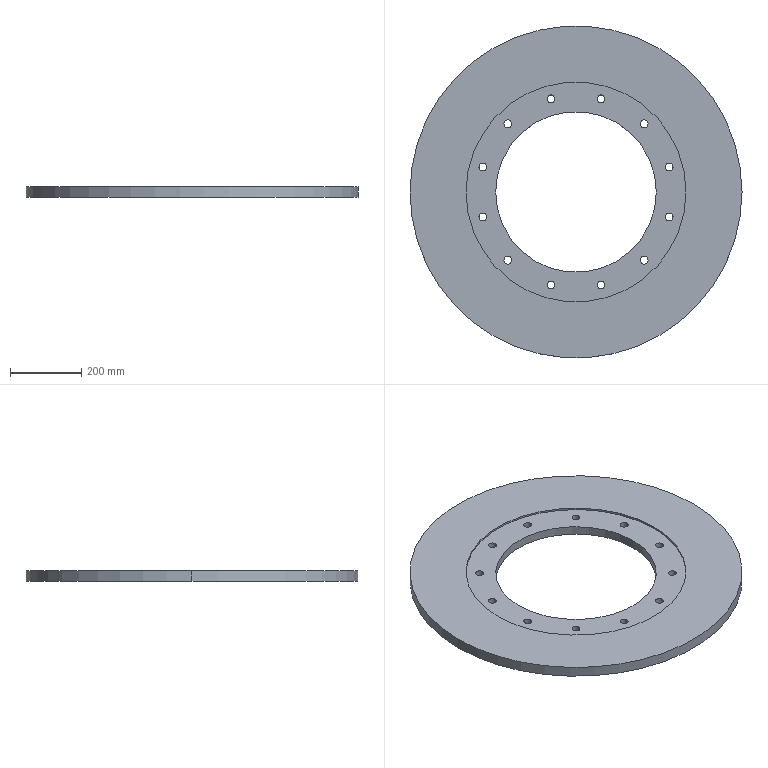Part | SolidWorks | features ICE 2, Extrusion 1 | 1 solid | 33 faces | box 930 x 930 x 30 mm | volume 14798488 mm3 | cylinder 30 | plane 3 | commonest cylinder face diameters 22 x24 450 x2 616 x2 930 x2
STEP:
#1=CARTESIAN_POINT('',(179.919,190.919,25.));
#2=VERTEX_POINT('',#1);
#3=CARTESIAN_POINT('',(201.919,190.919,25.));
#4=VERTEX_POINT('',#3);
#5=CARTESIAN_POINT('',(190.919,190.919,25.));
#6=DIRECTION('',(0.,0.,1.));
#7=DIRECTION('',(1.,0.,0.));
#8=AXIS2_PLACEMENT_3D('',#5,#6,#7);
#9=CIRCLE('',#8,11.);
#10=EDGE_CURVE('',#2,#4,#9,.T.);
#11=ORIENTED_EDGE('',*,*,#10,.T.);
#12=CARTESIAN_POINT('',(201.919,190.919,0.));
#13=VERTEX_POINT('',#12);
#14=CARTESIAN_POINT('',(201.919,190.919,30.));
#15=DIRECTION('',(0.,0.,-1.));
#16=VECTOR('',#15,1000.);
#17=LINE('',#14,#16);
#18=EDGE_CURVE('',#4,#13,#17,.T.);
#19=ORIENTED_EDGE('',*,*,#18,.T.);
#20=CARTESIAN_POINT('',(179.919,190.919,0.));
#21=VERTEX_POINT('',#20);
#22=CARTESIAN_POINT('',(190.919,190.919,0.));
#23=DIRECTION('',(0.,0.,1.));
#24=DIRECTION('',(1.,0.,0.));
#25=AXIS2_PLACEMENT_3D('',#22,#23,#24);
#26=CIRCLE('',#25,11.);
#27=EDGE_CURVE('',#21,#13,#26,.T.);
#28=ORIENTED_EDGE('',*,*,#27,.F.);
#29=CARTESIAN_POINT('',(179.919,190.919,30.));
#30=DIRECTION('',(0.,0.,-1.));
#31=VECTOR('',#30,1000.);
#32=LINE('',#29,#31);
#33=EDGE_CURVE('',#2,#21,#32,.T.);
#34=ORIENTED_EDGE('',*,*,#33,.F.);
#35=EDGE_LOOP('',(#11,#19,#28,#34));
#36=FACE_OUTER_BOUND('',#35,.T.);
#37=CARTESIAN_POINT('',(190.919,190.919,30.));
#38=DIRECTION('',(0.,0.,-1.));
#39=DIRECTION('',(-1.,0.,0.));
#40=AXIS2_PLACEMENT_3D('',#37,#38,#39);
#41=CYLINDRICAL_SURFACE('',#40,11.);
#42=ADVANCED_FACE('',(#36),#41,.F.);
#43=CARTESIAN_POINT('',(58.881,260.8,25.));
#44=VERTEX_POINT('',#43);
#45=CARTESIAN_POINT('',(80.881,260.8,25.));
#46=VERTEX_POINT('',#45);
#47=CARTESIAN_POINT('',(69.881,260.8,25.));
#48=DIRECTION('',(0.,0.,1.));
#49=DIRECTION('',(1.,0.,0.));
#50=AXIS2_PLACEMENT_3D('',#47,#48,#49);
#51=CIRCLE('',#50,11.);
#52=EDGE_CURVE('',#44,#46,#51,.T.);
#53=ORIENTED_EDGE('',*,*,#52,.T.);
#54=CARTESIAN_POINT('',(80.881,260.8,0.));
#55=VERTEX_POINT('',#54);
#56=CARTESIAN_POINT('',(80.881,260.8,30.));
#57=DIRECTION('',(0.,0.,-1.));
#58=VECTOR('',#57,1000.);
#59=LINE('',#56,#58);
#60=EDGE_CURVE('',#46,#55,#59,.T.);
#61=ORIENTED_EDGE('',*,*,#60,.T.);
#62=CARTESIAN_POINT('',(58.881,260.8,0.));
#63=VERTEX_POINT('',#62);
#64=CARTESIAN_POINT('',(69.881,260.8,0.));
#65=DIRECTION('',(0.,0.,1.));
#66=DIRECTION('',(1.,0.,0.));
#67=AXIS2_PLACEMENT_3D('',#64,#65,#66);
#68=CIRCLE('',#67,11.);
#69=EDGE_CURVE('',#63,#55,#68,.T.);
#70=ORIENTED_EDGE('',*,*,#69,.F.);
#71=CARTESIAN_POINT('',(58.881,260.8,30.));
#72=DIRECTION('',(0.,0.,-1.));
#73=VECTOR('',#72,1000.);
#74=LINE('',#71,#73);
#75=EDGE_CURVE('',#44,#63,#74,.T.);
#76=ORIENTED_EDGE('',*,*,#75,.F.);
#77=EDGE_LOOP('',(#53,#61,#70,#76));
#78=FACE_OUTER_BOUND('',#77,.T.);
#79=CARTESIAN_POINT('',(69.881,260.8,30.));
#80=DIRECTION('',(0.,0.,-1.));
#81=DIRECTION('',(-1.,0.,0.));
#82=AXIS2_PLACEMENT_3D('',#79,#80,#81);
#83=CYLINDRICAL_SURFACE('',#82,11.);
#84=ADVANCED_FACE('',(#78),#83,.F.);
#85=CARTESIAN_POINT('',(-80.881,260.8,25.));
#86=VERTEX_POINT('',#85);
#87=CARTESIAN_POINT('',(-58.881,260.8,25.));
#88=VERTEX_POINT('',#87);
#89=CARTESIAN_POINT('',(-69.881,260.8,25.));
#90=DIRECTION('',(0.,0.,1.));
#91=DIRECTION('',(1.,0.,0.));
#92=AXIS2_PLACEMENT_3D('',#89,#90,#91);
#93=CIRCLE('',#92,11.);
#94=EDGE_CURVE('',#86,#88,#93,.T.);
#95=ORIENTED_EDGE('',*,*,#94,.T.);
#96=CARTESIAN_POINT('',(-58.881,260.8,0.));
#97=VERTEX_POINT('',#96);
#98=CARTESIAN_POINT('',(-58.881,260.8,30.));
#99=DIRECTION('',(0.,0.,-1.));
#100=VECTOR('',#99,1000.);
#101=LINE('',#98,#100);
#102=EDGE_CURVE('',#88,#97,#101,.T.);
#103=ORIENTED_EDGE('',*,*,#102,.T.);
#104=CARTESIAN_POINT('',(-80.881,260.8,0.));
#105=VERTEX_POINT('',#104);
#106=CARTESIAN_POINT('',(-69.881,260.8,0.));
#107=DIRECTION('',(0.,0.,1.));
#108=DIRECTION('',(1.,0.,0.));
#109=AXIS2_PLACEMENT_3D('',#106,#107,#108);
#110=CIRCLE('',#109,11.);
#111=EDGE_CURVE('',#105,#97,#110,.T.);
#112=ORIENTED_EDGE('',*,*,#111,.F.);
#113=CARTESIAN_POINT('',(-80.881,260.8,30.));
#114=DIRECTION('',(0.,0.,-1.));
#115=VECTOR('',#114,1000.);
#116=LINE('',#113,#115);
#117=EDGE_CURVE('',#86,#105,#116,.T.);
#118=ORIENTED_EDGE('',*,*,#117,.F.);
#119=EDGE_LOOP('',(#95,#103,#112,#118));
#120=FACE_OUTER_BOUND('',#119,.T.);
#121=CARTESIAN_POINT('',(-69.881,260.8,30.));
#122=DIRECTION('',(0.,0.,-1.));
#123=DIRECTION('',(-1.,0.,0.));
#124=AXIS2_PLACEMENT_3D('',#121,#122,#123);
#125=CYLINDRICAL_SURFACE('',#124,11.);
#126=ADVANCED_FACE('',(#120),#125,.F.);
#127=CARTESIAN_POINT('',(-201.919,190.919,25.));
#128=VERTEX_POINT('',#127);
#129=CARTESIAN_POINT('',(-179.919,190.919,25.));
#130=VERTEX_POINT('',#129);
#131=CARTESIAN_POINT('',(-190.919,190.919,25.));
#132=DIRECTION('',(0.,0.,1.));
#133=DIRECTION('',(1.,0.,0.));
#134=AXIS2_PLACEMENT_3D('',#131,#132,#133);
#135=CIRCLE('',#134,11.);
#136=EDGE_CURVE('',#128,#130,#135,.T.);
#137=ORIENTED_EDGE('',*,*,#136,.T.);
#138=CARTESIAN_POINT('',(-179.919,190.919,0.));
#139=VERTEX_POINT('',#138);
#140=CARTESIAN_POINT('',(-179.919,190.919,30.));
#141=DIRECTION('',(0.,0.,-1.));
#142=VECTOR('',#141,1000.);
#143=LINE('',#140,#142);
#144=EDGE_CURVE('',#130,#139,#143,.T.);
#145=ORIENTED_EDGE('',*,*,#144,.T.);
#146=CARTESIAN_POINT('',(-201.919,190.919,0.));
#147=VERTEX_POINT('',#146);
#148=CARTESIAN_POINT('',(-190.919,190.919,0.));
#149=DIRECTION('',(0.,0.,1.));
#150=DIRECTION('',(1.,0.,0.));
#151=AXIS2_PLACEMENT_3D('',#148,#149,#150);
#152=CIRCLE('',#151,11.);
#153=EDGE_CURVE('',#147,#139,#152,.T.);
#154=ORIENTED_EDGE('',*,*,#153,.F.);
#155=CARTESIAN_POINT('',(-201.919,190.919,30.));
#156=DIRECTION('',(0.,0.,-1.));
#157=VECTOR('',#156,1000.);
#158=LINE('',#155,#157);
#159=EDGE_CURVE('',#128,#147,#158,.T.);
#160=ORIENTED_EDGE('',*,*,#159,.F.);
#161=EDGE_LOOP('',(#137,#145,#154,#160));
#162=FACE_OUTER_BOUND('',#161,.T.);
#163=CARTESIAN_POINT('',(-190.919,190.919,30.));
#164=DIRECTION('',(0.,0.,-1.));
#165=DIRECTION('',(-1.,0.,0.));
#166=AXIS2_PLACEMENT_3D('',#163,#164,#165);
#167=CYLINDRICAL_SURFACE('',#166,11.);
#168=ADVANCED_FACE('',(#162),#167,.F.);
#169=CARTESIAN_POINT('',(-271.8,69.881,25.));
#170=VERTEX_POINT('',#169);
#171=CARTESIAN_POINT('',(-249.8,69.881,25.));
#172=VERTEX_POINT('',#171);
#173=CARTESIAN_POINT('',(-260.8,69.881,25.));
#174=DIRECTION('',(0.,0.,1.));
#175=DIRECTION('',(1.,0.,0.));
#176=AXIS2_PLACEMENT_3D('',#173,#174,#175);
#177=CIRCLE('',#176,11.);
#178=EDGE_CURVE('',#170,#172,#177,.T.);
#179=ORIENTED_EDGE('',*,*,#178,.T.);
#180=CARTESIAN_POINT('',(-249.8,69.881,0.));
#181=VERTEX_POINT('',#180);
#182=CARTESIAN_POINT('',(-249.8,69.881,30.));
#183=DIRECTION('',(0.,0.,-1.));
#184=VECTOR('',#183,1000.);
#185=LINE('',#182,#184);
#186=EDGE_CURVE('',#172,#181,#185,.T.);
#187=ORIENTED_EDGE('',*,*,#186,.T.);
#188=CARTESIAN_POINT('',(-271.8,69.881,0.));
#189=VERTEX_POINT('',#188);
#190=CARTESIAN_POINT('',(-260.8,69.881,0.));
#191=DIRECTION('',(0.,0.,1.));
#192=DIRECTION('',(1.,0.,0.));
#193=AXIS2_PLACEMENT_3D('',#190,#191,#192);
#194=CIRCLE('',#193,11.);
#195=EDGE_CURVE('',#189,#181,#194,.T.);
#196=ORIENTED_EDGE('',*,*,#195,.F.);
#197=CARTESIAN_POINT('',(-271.8,69.881,30.));
#198=DIRECTION('',(0.,0.,-1.));
#199=VECTOR('',#198,1000.);
#200=LINE('',#197,#199);
#201=EDGE_CURVE('',#170,#189,#200,.T.);
#202=ORIENTED_EDGE('',*,*,#201,.F.);
#203=EDGE_LOOP('',(#179,#187,#196,#202));
#204=FACE_OUTER_BOUND('',#203,.T.);
#205=CARTESIAN_POINT('',(-260.8,69.881,30.));
#206=DIRECTION('',(0.,0.,-1.));
#207=DIRECTION('',(-1.,0.,0.));
#208=AXIS2_PLACEMENT_3D('',#205,#206,#207);
#209=CYLINDRICAL_SURFACE('',#208,11.);
#210=ADVANCED_FACE('',(#204),#209,.F.);
#211=CARTESIAN_POINT('',(-271.8,-69.881,25.));
#212=VERTEX_POINT('',#211);
#213=CARTESIAN_POINT('',(-249.8,-69.881,25.));
#214=VERTEX_POINT('',#213);
#215=CARTESIAN_POINT('',(-260.8,-69.881,25.));
#216=DIRECTION('',(0.,0.,1.));
#217=DIRECTION('',(1.,0.,0.));
#218=AXIS2_PLACEMENT_3D('',#215,#216,#217);
#219=CIRCLE('',#218,11.);
#220=EDGE_CURVE('',#212,#214,#219,.T.);
#221=ORIENTED_EDGE('',*,*,#220,.T.);
#222=CARTESIAN_POINT('',(-249.8,-69.881,0.));
#223=VERTEX_POINT('',#222);
#224=CARTESIAN_POINT('',(-249.8,-69.881,30.));
#225=DIRECTION('',(0.,0.,-1.));
#226=VECTOR('',#225,1000.);
#227=LINE('',#224,#226);
#228=EDGE_CURVE('',#214,#223,#227,.T.);
#229=ORIENTED_EDGE('',*,*,#228,.T.);
#230=CARTESIAN_POINT('',(-271.8,-69.881,0.));
#231=VERTEX_POINT('',#230);
#232=CARTESIAN_POINT('',(-260.8,-69.881,0.));
#233=DIRECTION('',(0.,0.,1.));
#234=DIRECTION('',(1.,0.,0.));
#235=AXIS2_PLACEMENT_3D('',#232,#233,#234);
#236=CIRCLE('',#235,11.);
#237=EDGE_CURVE('',#231,#223,#236,.T.);
#238=ORIENTED_EDGE('',*,*,#237,.F.);
#239=CARTESIAN_POINT('',(-271.8,-69.881,30.));
#240=DIRECTION('',(0.,0.,-1.));
#241=VECTOR('',#240,1000.);
#242=LINE('',#239,#241);
#243=EDGE_CURVE('',#212,#231,#242,.T.);
#244=ORIENTED_EDGE('',*,*,#243,.F.);
#245=EDGE_LOOP('',(#221,#229,#238,#244));
#246=FACE_OUTER_BOUND('',#245,.T.);
#247=CARTESIAN_POINT('',(-260.8,-69.881,30.));
#248=DIRECTION('',(0.,0.,-1.));
#249=DIRECTION('',(-1.,0.,0.));
#250=AXIS2_PLACEMENT_3D('',#247,#248,#249);
#251=CYLINDRICAL_SURFACE('',#250,11.);
#252=ADVANCED_FACE('',(#246),#251,.F.);
#253=CARTESIAN_POINT('',(-201.919,-190.919,25.));
#254=VERTEX_POINT('',#253);
#255=CARTESIAN_POINT('',(-179.919,-190.919,25.));
#256=VERTEX_POINT('',#255);
#257=CARTESIAN_POINT('',(-190.919,-190.919,25.));
#258=DIRECTION('',(0.,0.,1.));
#259=DIRECTION('',(1.,0.,0.));
#260=AXIS2_PLACEMENT_3D('',#257,#258,#259);
#261=CIRCLE('',#260,11.);
#262=EDGE_CURVE('',#254,#256,#261,.T.);
#263=ORIENTED_EDGE('',*,*,#262,.T.);
#264=CARTESIAN_POINT('',(-179.919,-190.919,0.));
#265=VERTEX_POINT('',#264);
#266=CARTESIAN_POINT('',(-179.919,-190.919,30.));
#267=DIRECTION('',(0.,0.,-1.));
#268=VECTOR('',#267,1000.);
#269=LINE('',#266,#268);
#270=EDGE_CURVE('',#256,#265,#269,.T.);
#271=ORIENTED_EDGE('',*,*,#270,.T.);
#272=CARTESIAN_POINT('',(-201.919,-190.919,0.));
#273=VERTEX_POINT('',#272);
#274=CARTESIAN_POINT('',(-190.919,-190.919,0.));
#275=DIRECTION('',(0.,0.,1.));
#276=DIRECTION('',(1.,0.,0.));
#277=AXIS2_PLACEMENT_3D('',#274,#275,#276);
#278=CIRCLE('',#277,11.);
#279=EDGE_CURVE('',#273,#265,#278,.T.);
#280=ORIENTED_EDGE('',*,*,#279,.F.);
#281=CARTESIAN_POINT('',(-201.919,-190.919,30.));
#282=DIRECTION('',(0.,0.,-1.));
#283=VECTOR('',#282,1000.);
#284=LINE('',#281,#283);
#285=EDGE_CURVE('',#254,#273,#284,.T.);
#286=ORIENTED_EDGE('',*,*,#285,.F.);
#287=EDGE_LOOP('',(#263,#271,#280,#286));
#288=FACE_OUTER_BOUND('',#287,.T.);
#289=CARTESIAN_POINT('',(-190.919,-190.919,30.));
#290=DIRECTION('',(0.,0.,-1.));
#291=DIRECTION('',(-1.,0.,0.));
#292=AXIS2_PLACEMENT_3D('',#289,#290,#291);
#293=CYLINDRICAL_SURFACE('',#292,11.);
#294=ADVANCED_FACE('',(#288),#293,.F.);
#295=CARTESIAN_POINT('',(-80.881,-260.8,25.));
#296=VERTEX_POINT('',#295);
#297=CARTESIAN_POINT('',(-58.881,-260.8,25.));
#298=VERTEX_POINT('',#297);
#299=CARTESIAN_POINT('',(-69.881,-260.8,25.));
#300=DIRECTION('',(0.,0.,1.));
#301=DIRECTION('',(1.,0.,0.));
#302=AXIS2_PLACEMENT_3D('',#299,#300,#301);
#303=CIRCLE('',#302,11.);
#304=EDGE_CURVE('',#296,#298,#303,.T.);
#305=ORIENTED_EDGE('',*,*,#304,.T.);
#306=CARTESIAN_POINT('',(-58.881,-260.8,0.));
#307=VERTEX_POINT('',#306);
#308=CARTESIAN_POINT('',(-58.881,-260.8,30.));
#309=DIRECTION('',(0.,0.,-1.));
#310=VECTOR('',#309,1000.);
#311=LINE('',#308,#310);
#312=EDGE_CURVE('',#298,#307,#311,.T.);
#313=ORIENTED_EDGE('',*,*,#312,.T.);
#314=CARTESIAN_POINT('',(-80.881,-260.8,0.));
#315=VERTEX_POINT('',#314);
#316=CARTESIAN_POINT('',(-69.881,-260.8,0.));
#317=DIRECTION('',(0.,0.,1.));
#318=DIRECTION('',(1.,0.,0.));
#319=AXIS2_PLACEMENT_3D('',#316,#317,#318);
#320=CIRCLE('',#319,11.);
#321=EDGE_CURVE('',#315,#307,#320,.T.);
#322=ORIENTED_EDGE('',*,*,#321,.F.);
#323=CARTESIAN_POINT('',(-80.881,-260.8,30.));
#324=DIRECTION('',(0.,0.,-1.));
#325=VECTOR('',#324,1000.);
#326=LINE('',#323,#325);
#327=EDGE_CURVE('',#296,#315,#326,.T.);
#328=ORIENTED_EDGE('',*,*,#327,.F.);
#329=EDGE_LOOP('',(#305,#313,#322,#328));
#330=FACE_OUTER_BOUND('',#329,.T.);
#331=CARTESIAN_POINT('',(-69.881,-260.8,30.));
#332=DIRECTION('',(0.,0.,-1.));
#333=DIRECTION('',(-1.,0.,0.));
#334=AXIS2_PLACEMENT_3D('',#331,#332,#333);
#335=CYLINDRICAL_SURFACE('',#334,11.);
#336=ADVANCED_FACE('',(#330),#335,.F.);
#337=CARTESIAN_POINT('',(58.881,-260.8,25.));
#338=VERTEX_POINT('',#337);
#339=CARTESIAN_POINT('',(80.881,-260.8,25.));
#340=VERTEX_POINT('',#339);
#341=CARTESIAN_POINT('',(69.881,-260.8,25.));
#342=DIRECTION('',(0.,0.,1.));
#343=DIRECTION('',(1.,0.,0.));
#344=AXIS2_PLACEMENT_3D('',#341,#342,#343);
#345=CIRCLE('',#344,11.);
#346=EDGE_CURVE('',#338,#340,#345,.T.);
#347=ORIENTED_EDGE('',*,*,#346,.T.);
#348=CARTESIAN_POINT('',(80.881,-260.8,0.));
#349=VERTEX_POINT('',#348);
#350=CARTESIAN_POINT('',(80.881,-260.8,30.));
#351=DIRECTION('',(0.,0.,-1.));
#352=VECTOR('',#351,1000.);
#353=LINE('',#350,#352);
#354=EDGE_CURVE('',#340,#349,#353,.T.);
#355=ORIENTED_EDGE('',*,*,#354,.T.);
#356=CARTESIAN_POINT('',(58.881,-260.8,0.));
#357=VERTEX_POINT('',#356);
#358=CARTESIAN_POINT('',(69.881,-260.8,0.));
#359=DIRECTION('',(0.,0.,1.));
#360=DIRECTION('',(1.,0.,0.));
#361=AXIS2_PLACEMENT_3D('',#358,#359,#360);
#362=CIRCLE('',#361,11.);
#363=EDGE_CURVE('',#357,#349,#362,.T.);
#364=ORIENTED_EDGE('',*,*,#363,.F.);
#365=CARTESIAN_POINT('',(58.881,-260.8,30.));
#366=DIRECTION('',(0.,0.,-1.));
#367=VECTOR('',#366,1000.);
#368=LINE('',#365,#367);
#369=EDGE_CURVE('',#338,#357,#368,.T.);
#370=ORIENTED_EDGE('',*,*,#369,.F.);
#371=EDGE_LOOP('',(#347,#355,#364,#370));
#372=FACE_OUTER_BOUND('',#371,.T.);
#373=CARTESIAN_POINT('',(69.881,-260.8,30.));
#374=DIRECTION('',(0.,0.,-1.));
#375=DIRECTION('',(-1.,0.,0.));
#376=AXIS2_PLACEMENT_3D('',#373,#374,#375);
#377=CYLINDRICAL_SURFACE('',#376,11.);
#378=ADVANCED_FACE('',(#372),#377,.F.);
#379=CARTESIAN_POINT('',(179.919,-190.919,25.));
#380=VERTEX_POINT('',#379);
#381=CARTESIAN_POINT('',(201.919,-190.919,25.));
#382=VERTEX_POINT('',#381);
#383=CARTESIAN_POINT('',(190.919,-190.919,25.));
#384=DIRECTION('',(0.,0.,1.));
#385=DIRECTION('',(1.,0.,0.));
#386=AXIS2_PLACEMENT_3D('',#383,#384,#385);
#387=CIRCLE('',#386,11.);
#388=EDGE_CURVE('',#380,#382,#387,.T.);
#389=ORIENTED_EDGE('',*,*,#388,.T.);
#390=CARTESIAN_POINT('',(201.919,-190.919,0.));
#391=VERTEX_POINT('',#390);
#392=CARTESIAN_POINT('',(201.919,-190.919,30.));
#393=DIRECTION('',(0.,0.,-1.));
#394=VECTOR('',#393,1000.);
#395=LINE('',#392,#394);
#396=EDGE_CURVE('',#382,#391,#395,.T.);
#397=ORIENTED_EDGE('',*,*,#396,.T.);
#398=CARTESIAN_POINT('',(179.919,-190.919,0.));
#399=VERTEX_POINT('',#398);
#400=CARTESIAN_POINT('',(190.919,-190.919,0.));
#401=DIRECTION('',(0.,0.,1.));
#402=DIRECTION('',(1.,0.,0.));
#403=AXIS2_PLACEMENT_3D('',#400,#401,#402);
#404=CIRCLE('',#403,11.);
#405=EDGE_CURVE('',#399,#391,#404,.T.);
#406=ORIENTED_EDGE('',*,*,#405,.F.);
#407=CARTESIAN_POINT('',(179.919,-190.919,30.));
#408=DIRECTION('',(0.,0.,-1.));
#409=VECTOR('',#408,1000.);
#410=LINE('',#407,#409);
#411=EDGE_CURVE('',#380,#399,#410,.T.);
#412=ORIENTED_EDGE('',*,*,#411,.F.);
#413=EDGE_LOOP('',(#389,#397,#406,#412));
#414=FACE_OUTER_BOUND('',#413,.T.);
#415=CARTESIAN_POINT('',(190.919,-190.919,30.));
#416=DIRECTION('',(0.,0.,-1.));
#417=DIRECTION('',(-1.,0.,0.));
#418=AXIS2_PLACEMENT_3D('',#415,#416,#417);
#419=CYLINDRICAL_SURFACE('',#418,11.);
#420=ADVANCED_FACE('',(#414),#419,.F.);
#421=CARTESIAN_POINT('',(249.8,-69.881,25.));
#422=VERTEX_POINT('',#421);
#423=CARTESIAN_POINT('',(271.8,-69.881,25.));
#424=VERTEX_POINT('',#423);
#425=CARTESIAN_POINT('',(260.8,-69.881,25.));
#426=DIRECTION('',(0.,0.,1.));
#427=DIRECTION('',(1.,0.,0.));
#428=AXIS2_PLACEMENT_3D('',#425,#426,#427);
#429=CIRCLE('',#428,11.);
#430=EDGE_CURVE('',#422,#424,#429,.T.);
#431=ORIENTED_EDGE('',*,*,#430,.T.);
#432=CARTESIAN_POINT('',(271.8,-69.881,0.));
#433=VERTEX_POINT('',#432);
#434=CARTESIAN_POINT('',(271.8,-69.881,30.));
#435=DIRECTION('',(0.,0.,-1.));
#436=VECTOR('',#435,1000.);
#437=LINE('',#434,#436);
#438=EDGE_CURVE('',#424,#433,#437,.T.);
#439=ORIENTED_EDGE('',*,*,#438,.T.);
#440=CARTESIAN_POINT('',(249.8,-69.881,0.));
#441=VERTEX_POINT('',#440);
#442=CARTESIAN_POINT('',(260.8,-69.881,0.));
#443=DIRECTION('',(0.,0.,1.));
#444=DIRECTION('',(1.,0.,0.));
#445=AXIS2_PLACEMENT_3D('',#442,#443,#444);
#446=CIRCLE('',#445,11.);
#447=EDGE_CURVE('',#441,#433,#446,.T.);
#448=ORIENTED_EDGE('',*,*,#447,.F.);
#449=CARTESIAN_POINT('',(249.8,-69.881,30.));
#450=DIRECTION('',(0.,0.,-1.));
#451=VECTOR('',#450,1000.);
#452=LINE('',#449,#451);
#453=EDGE_CURVE('',#422,#441,#452,.T.);
#454=ORIENTED_EDGE('',*,*,#453,.F.);
#455=EDGE_LOOP('',(#431,#439,#448,#454));
#456=FACE_OUTER_BOUND('',#455,.T.);
#457=CARTESIAN_POINT('',(260.8,-69.881,30.));
#458=DIRECTION('',(0.,0.,-1.));
#459=DIRECTION('',(-1.,0.,0.));
#460=AXIS2_PLACEMENT_3D('',#457,#458,#459);
#461=CYLINDRICAL_SURFACE('',#460,11.);
#462=ADVANCED_FACE('',(#456),#461,.F.);
#463=CARTESIAN_POINT('',(249.8,69.881,25.));
#464=VERTEX_POINT('',#463);
#465=CARTESIAN_POINT('',(271.8,69.881,25.));
#466=VERTEX_POINT('',#465);
#467=CARTESIAN_POINT('',(260.8,69.881,25.));
#468=DIRECTION('',(0.,0.,1.));
#469=DIRECTION('',(1.,0.,0.));
#470=AXIS2_PLACEMENT_3D('',#467,#468,#469);
#471=CIRCLE('',#470,11.);
#472=EDGE_CURVE('',#464,#466,#471,.T.);
#473=ORIENTED_EDGE('',*,*,#472,.T.);
#474=CARTESIAN_POINT('',(271.8,69.881,0.));
#475=VERTEX_POINT('',#474);
#476=CARTESIAN_POINT('',(271.8,69.881,30.));
#477=DIRECTION('',(0.,0.,-1.));
#478=VECTOR('',#477,1000.);
#479=LINE('',#476,#478);
#480=EDGE_CURVE('',#466,#475,#479,.T.);
#481=ORIENTED_EDGE('',*,*,#480,.T.);
#482=CARTESIAN_POINT('',(249.8,69.881,0.));
#483=VERTEX_POINT('',#482);
#484=CARTESIAN_POINT('',(260.8,69.881,0.));
#485=DIRECTION('',(0.,0.,1.));
#486=DIRECTION('',(1.,0.,0.));
#487=AXIS2_PLACEMENT_3D('',#484,#485,#486);
#488=CIRCLE('',#487,11.);
#489=EDGE_CURVE('',#483,#475,#488,.T.);
#490=ORIENTED_EDGE('',*,*,#489,.F.);
#491=CARTESIAN_POINT('',(249.8,69.881,30.));
#492=DIRECTION('',(0.,0.,-1.));
#493=VECTOR('',#492,1000.);
#494=LINE('',#491,#493);
#495=EDGE_CURVE('',#464,#483,#494,.T.);
#496=ORIENTED_EDGE('',*,*,#495,.F.);
#497=EDGE_LOOP('',(#473,#481,#490,#496));
#498=FACE_OUTER_BOUND('',#497,.T.);
#499=CARTESIAN_POINT('',(260.8,69.881,30.));
#500=DIRECTION('',(0.,0.,-1.));
#501=DIRECTION('',(-1.,0.,0.));
#502=AXIS2_PLACEMENT_3D('',#499,#500,#501);
#503=CYLINDRICAL_SURFACE('',#502,11.);
#504=ADVANCED_FACE('',(#498),#503,.F.);
#505=CARTESIAN_POINT('',(-308.,0.,25.));
#506=VERTEX_POINT('',#505);
#507=CARTESIAN_POINT('',(308.,0.,25.));
#508=VERTEX_POINT('',#507);
#509=CARTESIAN_POINT('',(0.,0.,25.));
#510=DIRECTION('',(0.,0.,1.));
#511=DIRECTION('',(1.,0.,0.));
#512=AXIS2_PLACEMENT_3D('',#509,#510,#511);
#513=CIRCLE('',#512,308.);
#514=EDGE_CURVE('',#506,#508,#513,.T.);
#515=ORIENTED_EDGE('',*,*,#514,.F.);
#516=CARTESIAN_POINT('',(-308.,0.,30.));
#517=VERTEX_POINT('',#516);
#518=CARTESIAN_POINT('',(-308.,0.,25.));
#519=DIRECTION('',(0.,0.,1.));
#520=VECTOR('',#519,1000.);
#521=LINE('',#518,#520);
#522=EDGE_CURVE('',#506,#517,#521,.T.);
#523=ORIENTED_EDGE('',*,*,#522,.T.);
#524=CARTESIAN_POINT('',(308.,0.,30.));
#525=VERTEX_POINT('',#524);
#526=CARTESIAN_POINT('',(0.,0.,30.));
#527=DIRECTION('',(0.,0.,1.));
#528=DIRECTION('',(1.,0.,0.));
#529=AXIS2_PLACEMENT_3D('',#526,#527,#528);
#530=CIRCLE('',#529,308.);
#531=EDGE_CURVE('',#517,#525,#530,.T.);
#532=ORIENTED_EDGE('',*,*,#531,.T.);
#533=CARTESIAN_POINT('',(308.,0.,25.));
#534=DIRECTION('',(0.,0.,1.));
#535=VECTOR('',#534,1000.);
#536=LINE('',#533,#535);
#537=EDGE_CURVE('',#508,#525,#536,.T.);
#538=ORIENTED_EDGE('',*,*,#537,.F.);
#539=EDGE_LOOP('',(#515,#523,#532,#538));
#540=FACE_OUTER_BOUND('',#539,.T.);
#541=CARTESIAN_POINT('',(0.,0.,25.));
#542=DIRECTION('',(0.,0.,1.));
#543=DIRECTION('',(1.,0.,0.));
#544=AXIS2_PLACEMENT_3D('',#541,#542,#543);
#545=CYLINDRICAL_SURFACE('',#544,308.);
#546=ADVANCED_FACE('',(#540),#545,.F.);
#547=CARTESIAN_POINT('',(465.,0.,30.));
#548=VERTEX_POINT('',#547);
#549=CARTESIAN_POINT('',(-465.,0.,30.));
#550=VERTEX_POINT('',#549);
#551=CARTESIAN_POINT('',(0.,0.,30.));
#552=DIRECTION('',(0.,0.,1.));
#553=DIRECTION('',(1.,0.,0.));
#554=AXIS2_PLACEMENT_3D('',#551,#552,#553);
#555=CIRCLE('',#554,465.);
#556=EDGE_CURVE('',#548,#550,#555,.T.);
#557=ORIENTED_EDGE('',*,*,#556,.F.);
#558=CARTESIAN_POINT('',(465.,0.,0.));
#559=VERTEX_POINT('',#558);
#560=CARTESIAN_POINT('',(465.,0.,30.));
#561=DIRECTION('',(0.,0.,-1.));
#562=VECTOR('',#561,1000.);
#563=LINE('',#560,#562);
#564=EDGE_CURVE('',#548,#559,#563,.T.);
#565=ORIENTED_EDGE('',*,*,#564,.T.);
#566=CARTESIAN_POINT('',(-465.,0.,0.));
#567=VERTEX_POINT('',#566);
#568=CARTESIAN_POINT('',(0.,0.,0.));
#569=DIRECTION('',(0.,0.,1.));
#570=DIRECTION('',(1.,0.,0.));
#571=AXIS2_PLACEMENT_3D('',#568,#569,#570);
#572=CIRCLE('',#571,465.);
#573=EDGE_CURVE('',#559,#567,#572,.T.);
#574=ORIENTED_EDGE('',*,*,#573,.T.);
#575=CARTESIAN_POINT('',(-465.,0.,30.));
#576=DIRECTION('',(0.,0.,-1.));
#577=VECTOR('',#576,1000.);
#578=LINE('',#575,#577);
#579=EDGE_CURVE('',#550,#567,#578,.T.);
#580=ORIENTED_EDGE('',*,*,#579,.F.);
#581=EDGE_LOOP('',(#557,#565,#574,#580));
#582=FACE_OUTER_BOUND('',#581,.T.);
#583=CARTESIAN_POINT('',(0.,0.,30.));
#584=DIRECTION('',(0.,0.,-1.));
#585=DIRECTION('',(-1.,0.,0.));
#586=AXIS2_PLACEMENT_3D('',#583,#584,#585);
#587=CYLINDRICAL_SURFACE('',#586,465.);
#588=ADVANCED_FACE('',(#582),#587,.T.);
#589=CARTESIAN_POINT('',(-225.,0.,25.));
#590=VERTEX_POINT('',#589);
#591=CARTESIAN_POINT('',(225.,0.,25.));
#592=VERTEX_POINT('',#591);
#593=CARTESIAN_POINT('',(0.,0.,25.));
#594=DIRECTION('',(0.,0.,1.));
#595=DIRECTION('',(1.,0.,0.));
#596=AXIS2_PLACEMENT_3D('',#593,#594,#595);
#597=CIRCLE('',#596,225.);
#598=EDGE_CURVE('',#590,#592,#597,.T.);
#599=ORIENTED_EDGE('',*,*,#598,.T.);
#600=CARTESIAN_POINT('',(225.,0.,0.));
#601=VERTEX_POINT('',#600);
#602=CARTESIAN_POINT('',(225.,0.,30.));
#603=DIRECTION('',(0.,0.,-1.));
#604=VECTOR('',#603,1000.);
#605=LINE('',#602,#604);
#606=EDGE_CURVE('',#592,#601,#605,.T.);
#607=ORIENTED_EDGE('',*,*,#606,.T.);
#608=CARTESIAN_POINT('',(-225.,0.,0.));
#609=VERTEX_POINT('',#608);
#610=CARTESIAN_POINT('',(0.,0.,0.));
#611=DIRECTION('',(0.,0.,1.));
#612=DIRECTION('',(1.,0.,0.));
#613=AXIS2_PLACEMENT_3D('',#610,#611,#612);
#614=CIRCLE('',#613,225.);
#615=EDGE_CURVE('',#609,#601,#614,.T.);
#616=ORIENTED_EDGE('',*,*,#615,.F.);
#617=CARTESIAN_POINT('',(-225.,0.,30.));
#618=DIRECTION('',(0.,0.,-1.));
#619=VECTOR('',#618,1000.);
#620=LINE('',#617,#619);
#621=EDGE_CURVE('',#590,#609,#620,.T.);
#622=ORIENTED_EDGE('',*,*,#621,.F.);
#623=EDGE_LOOP('',(#599,#607,#616,#622));
#624=FACE_OUTER_BOUND('',#623,.T.);
#625=CARTESIAN_POINT('',(0.,0.,30.));
#626=DIRECTION('',(0.,0.,-1.));
#627=DIRECTION('',(-1.,0.,0.));
#628=AXIS2_PLACEMENT_3D('',#625,#626,#627);
#629=CYLINDRICAL_SURFACE('',#628,225.);
#630=ADVANCED_FACE('',(#624),#629,.F.);
#631=ORIENTED_EDGE('',*,*,#606,.F.);
#632=CARTESIAN_POINT('',(0.,0.,25.));
#633=DIRECTION('',(0.,0.,1.));
#634=DIRECTION('',(1.,0.,0.));
#635=AXIS2_PLACEMENT_3D('',#632,#633,#634);
#636=CIRCLE('',#635,225.);
#637=EDGE_CURVE('',#592,#590,#636,.T.);
#638=ORIENTED_EDGE('',*,*,#637,.T.);
#639=ORIENTED_EDGE('',*,*,#621,.T.);
#640=CARTESIAN_POINT('',(0.,0.,0.));
#641=DIRECTION('',(0.,0.,1.));
#642=DIRECTION('',(1.,0.,0.));
#643=AXIS2_PLACEMENT_3D('',#640,#641,#642);
#644=CIRCLE('',#643,225.);
#645=EDGE_CURVE('',#601,#609,#644,.T.);
#646=ORIENTED_EDGE('',*,*,#645,.F.);
#647=EDGE_LOOP('',(#631,#638,#639,#646));
#648=FACE_OUTER_BOUND('',#647,.T.);
#649=CARTESIAN_POINT('',(0.,0.,30.));
#650=DIRECTION('',(0.,0.,-1.));
#651=DIRECTION('',(-1.,0.,0.));
#652=AXIS2_PLACEMENT_3D('',#649,#650,#651);
#653=CYLINDRICAL_SURFACE('',#652,225.);
#654=ADVANCED_FACE('',(#648),#653,.F.);
#655=CARTESIAN_POINT('',(0.,0.,30.));
#656=DIRECTION('',(0.,0.,1.));
#657=DIRECTION('',(1.,0.,0.));
#658=AXIS2_PLACEMENT_3D('',#655,#656,#657);
#659=CIRCLE('',#658,308.);
#660=EDGE_CURVE('',#525,#517,#659,.T.);
#661=ORIENTED_EDGE('',*,*,#660,.F.);
#662=ORIENTED_EDGE('',*,*,#531,.F.);
#663=EDGE_LOOP('',(#661,#662));
#664=FACE_BOUND('',#663,.T.);
#665=CARTESIAN_POINT('',(0.,0.,30.));
#666=DIRECTION('',(0.,0.,1.));
#667=DIRECTION('',(1.,0.,0.));
#668=AXIS2_PLACEMENT_3D('',#665,#666,#667);
#669=CIRCLE('',#668,465.);
#670=EDGE_CURVE('',#550,#548,#669,.T.);
#671=ORIENTED_EDGE('',*,*,#670,.T.);
#672=ORIENTED_EDGE('',*,*,#556,.T.);
#673=EDGE_LOOP('',(#671,#672));
#674=FACE_OUTER_BOUND('',#673,.T.);
#675=CARTESIAN_POINT('',(0.,0.,30.));
#676=DIRECTION('',(0.,0.,1.));
#677=DIRECTION('',(1.,0.,0.));
#678=AXIS2_PLACEMENT_3D('',#675,#676,#677);
#679=PLANE('',#678);
#680=ADVANCED_FACE('',(#664,#674),#679,.T.);
#681=ORIENTED_EDGE('',*,*,#27,.T.);
#682=CARTESIAN_POINT('',(190.919,190.919,0.));
#683=DIRECTION('',(0.,0.,1.));
#684=DIRECTION('',(1.,0.,0.));
#685=AXIS2_PLACEMENT_3D('',#682,#683,#684);
#686=CIRCLE('',#685,11.);
#687=EDGE_CURVE('',#13,#21,#686,.T.);
#688=ORIENTED_EDGE('',*,*,#687,.T.);
#689=EDGE_LOOP('',(#681,#688));
#690=FACE_BOUND('',#689,.T.);
#691=ORIENTED_EDGE('',*,*,#69,.T.);
#692=CARTESIAN_POINT('',(69.881,260.8,0.));
#693=DIRECTION('',(0.,0.,1.));
#694=DIRECTION('',(1.,0.,0.));
#695=AXIS2_PLACEMENT_3D('',#692,#693,#694);
#696=CIRCLE('',#695,11.);
#697=EDGE_CURVE('',#55,#63,#696,.T.);
#698=ORIENTED_EDGE('',*,*,#697,.T.);
#699=EDGE_LOOP('',(#691,#698));
#700=FACE_BOUND('',#699,.T.);
#701=ORIENTED_EDGE('',*,*,#111,.T.);
#702=CARTESIAN_POINT('',(-69.881,260.8,0.));
#703=DIRECTION('',(0.,0.,1.));
#704=DIRECTION('',(1.,0.,0.));
#705=AXIS2_PLACEMENT_3D('',#702,#703,#704);
#706=CIRCLE('',#705,11.);
#707=EDGE_CURVE('',#97,#105,#706,.T.);
#708=ORIENTED_EDGE('',*,*,#707,.T.);
#709=EDGE_LOOP('',(#701,#708));
#710=FACE_BOUND('',#709,.T.);
#711=ORIENTED_EDGE('',*,*,#153,.T.);
#712=CARTESIAN_POINT('',(-190.919,190.919,0.));
#713=DIRECTION('',(0.,0.,1.));
#714=DIRECTION('',(1.,0.,0.));
#715=AXIS2_PLACEMENT_3D('',#712,#713,#714);
#716=CIRCLE('',#715,11.);
#717=EDGE_CURVE('',#139,#147,#716,.T.);
#718=ORIENTED_EDGE('',*,*,#717,.T.);
#719=EDGE_LOOP('',(#711,#718));
#720=FACE_BOUND('',#719,.T.);
#721=ORIENTED_EDGE('',*,*,#195,.T.);
#722=CARTESIAN_POINT('',(-260.8,69.881,0.));
#723=DIRECTION('',(0.,0.,1.));
#724=DIRECTION('',(1.,0.,0.));
#725=AXIS2_PLACEMENT_3D('',#722,#723,#724);
#726=CIRCLE('',#725,11.);
#727=EDGE_CURVE('',#181,#189,#726,.T.);
#728=ORIENTED_EDGE('',*,*,#727,.T.);
#729=EDGE_LOOP('',(#721,#728));
#730=FACE_BOUND('',#729,.T.);
#731=ORIENTED_EDGE('',*,*,#237,.T.);
#732=CARTESIAN_POINT('',(-260.8,-69.881,0.));
#733=DIRECTION('',(0.,0.,1.));
#734=DIRECTION('',(1.,0.,0.));
#735=AXIS2_PLACEMENT_3D('',#732,#733,#734);
#736=CIRCLE('',#735,11.);
#737=EDGE_CURVE('',#223,#231,#736,.T.);
#738=ORIENTED_EDGE('',*,*,#737,.T.);
#739=EDGE_LOOP('',(#731,#738));
#740=FACE_BOUND('',#739,.T.);
#741=ORIENTED_EDGE('',*,*,#279,.T.);
#742=CARTESIAN_POINT('',(-190.919,-190.919,0.));
#743=DIRECTION('',(0.,0.,1.));
#744=DIRECTION('',(1.,0.,0.));
#745=AXIS2_PLACEMENT_3D('',#742,#743,#744);
#746=CIRCLE('',#745,11.);
#747=EDGE_CURVE('',#265,#273,#746,.T.);
#748=ORIENTED_EDGE('',*,*,#747,.T.);
#749=EDGE_LOOP('',(#741,#748));
#750=FACE_BOUND('',#749,.T.);
#751=ORIENTED_EDGE('',*,*,#321,.T.);
#752=CARTESIAN_POINT('',(-69.881,-260.8,0.));
#753=DIRECTION('',(0.,0.,1.));
#754=DIRECTION('',(1.,0.,0.));
#755=AXIS2_PLACEMENT_3D('',#752,#753,#754);
#756=CIRCLE('',#755,11.);
#757=EDGE_CURVE('',#307,#315,#756,.T.);
#758=ORIENTED_EDGE('',*,*,#757,.T.);
#759=EDGE_LOOP('',(#751,#758));
#760=FACE_BOUND('',#759,.T.);
#761=ORIENTED_EDGE('',*,*,#363,.T.);
#762=CARTESIAN_POINT('',(69.881,-260.8,0.));
#763=DIRECTION('',(0.,0.,1.));
#764=DIRECTION('',(1.,0.,0.));
#765=AXIS2_PLACEMENT_3D('',#762,#763,#764);
#766=CIRCLE('',#765,11.);
#767=EDGE_CURVE('',#349,#357,#766,.T.);
#768=ORIENTED_EDGE('',*,*,#767,.T.);
#769=EDGE_LOOP('',(#761,#768));
#770=FACE_BOUND('',#769,.T.);
#771=ORIENTED_EDGE('',*,*,#405,.T.);
#772=CARTESIAN_POINT('',(190.919,-190.919,0.));
#773=DIRECTION('',(0.,0.,1.));
#774=DIRECTION('',(1.,0.,0.));
#775=AXIS2_PLACEMENT_3D('',#772,#773,#774);
#776=CIRCLE('',#775,11.);
#777=EDGE_CURVE('',#391,#399,#776,.T.);
#778=ORIENTED_EDGE('',*,*,#777,.T.);
#779=EDGE_LOOP('',(#771,#778));
#780=FACE_BOUND('',#779,.T.);
#781=ORIENTED_EDGE('',*,*,#447,.T.);
#782=CARTESIAN_POINT('',(260.8,-69.881,0.));
#783=DIRECTION('',(0.,0.,1.));
#784=DIRECTION('',(1.,0.,0.));
#785=AXIS2_PLACEMENT_3D('',#782,#783,#784);
#786=CIRCLE('',#785,11.);
#787=EDGE_CURVE('',#433,#441,#786,.T.);
#788=ORIENTED_EDGE('',*,*,#787,.T.);
#789=EDGE_LOOP('',(#781,#788));
#790=FACE_BOUND('',#789,.T.);
#791=ORIENTED_EDGE('',*,*,#489,.T.);
#792=CARTESIAN_POINT('',(260.8,69.881,0.));
#793=DIRECTION('',(0.,0.,1.));
#794=DIRECTION('',(1.,0.,0.));
#795=AXIS2_PLACEMENT_3D('',#792,#793,#794);
#796=CIRCLE('',#795,11.);
#797=EDGE_CURVE('',#475,#483,#796,.T.);
#798=ORIENTED_EDGE('',*,*,#797,.T.);
#799=EDGE_LOOP('',(#791,#798));
#800=FACE_BOUND('',#799,.T.);
#801=CARTESIAN_POINT('',(0.,0.,0.));
#802=DIRECTION('',(0.,0.,1.));
#803=DIRECTION('',(1.,0.,0.));
#804=AXIS2_PLACEMENT_3D('',#801,#802,#803);
#805=CIRCLE('',#804,465.);
#806=EDGE_CURVE('',#567,#559,#805,.T.);
#807=ORIENTED_EDGE('',*,*,#806,.F.);
#808=ORIENTED_EDGE('',*,*,#573,.F.);
#809=EDGE_LOOP('',(#807,#808));
#810=FACE_OUTER_BOUND('',#809,.T.);
#811=ORIENTED_EDGE('',*,*,#615,.T.);
#812=ORIENTED_EDGE('',*,*,#645,.T.);
#813=EDGE_LOOP('',(#811,#812));
#814=FACE_BOUND('',#813,.T.);
#815=CARTESIAN_POINT('',(0.,0.,0.));
#816=DIRECTION('',(0.,0.,1.));
#817=DIRECTION('',(1.,0.,0.));
#818=AXIS2_PLACEMENT_3D('',#815,#816,#817);
#819=PLANE('',#818);
#820=ADVANCED_FACE('',(#690,#700,#710,#720,#730,#740,#750,#760,#770,#780,#790,#800,#810,#814),#819,.F.);
#821=ORIENTED_EDGE('',*,*,#564,.F.);
#822=ORIENTED_EDGE('',*,*,#670,.F.);
#823=ORIENTED_EDGE('',*,*,#579,.T.);
#824=ORIENTED_EDGE('',*,*,#806,.T.);
#825=EDGE_LOOP('',(#821,#822,#823,#824));
#826=FACE_OUTER_BOUND('',#825,.T.);
#827=CARTESIAN_POINT('',(0.,0.,30.));
#828=DIRECTION('',(0.,0.,-1.));
#829=DIRECTION('',(-1.,0.,0.));
#830=AXIS2_PLACEMENT_3D('',#827,#828,#829);
#831=CYLINDRICAL_SURFACE('',#830,465.);
#832=ADVANCED_FACE('',(#826),#831,.T.);
#833=ORIENTED_EDGE('',*,*,#522,.F.);
#834=CARTESIAN_POINT('',(0.,0.,25.));
#835=DIRECTION('',(0.,0.,1.));
#836=DIRECTION('',(1.,0.,0.));
#837=AXIS2_PLACEMENT_3D('',#834,#835,#836);
#838=CIRCLE('',#837,308.);
#839=EDGE_CURVE('',#508,#506,#838,.T.);
#840=ORIENTED_EDGE('',*,*,#839,.F.);
#841=ORIENTED_EDGE('',*,*,#537,.T.);
#842=ORIENTED_EDGE('',*,*,#660,.T.);
#843=EDGE_LOOP('',(#833,#840,#841,#842));
#844=FACE_OUTER_BOUND('',#843,.T.);
#845=CARTESIAN_POINT('',(0.,0.,25.));
#846=DIRECTION('',(0.,0.,1.));
#847=DIRECTION('',(1.,0.,0.));
#848=AXIS2_PLACEMENT_3D('',#845,#846,#847);
#849=CYLINDRICAL_SURFACE('',#848,308.);
#850=ADVANCED_FACE('',(#844),#849,.F.);
#851=ORIENTED_EDGE('',*,*,#10,.F.);
#852=CARTESIAN_POINT('',(190.919,190.919,25.));
#853=DIRECTION('',(0.,0.,1.));
#854=DIRECTION('',(1.,0.,0.));
#855=AXIS2_PLACEMENT_3D('',#852,#853,#854);
#856=CIRCLE('',#855,11.);
#857=EDGE_CURVE('',#4,#2,#856,.T.);
#858=ORIENTED_EDGE('',*,*,#857,.F.);
#859=EDGE_LOOP('',(#851,#858));
#860=FACE_BOUND('',#859,.T.);
#861=ORIENTED_EDGE('',*,*,#52,.F.);
#862=CARTESIAN_POINT('',(69.881,260.8,25.));
#863=DIRECTION('',(0.,0.,1.));
#864=DIRECTION('',(1.,0.,0.));
#865=AXIS2_PLACEMENT_3D('',#862,#863,#864);
#866=CIRCLE('',#865,11.);
#867=EDGE_CURVE('',#46,#44,#866,.T.);
#868=ORIENTED_EDGE('',*,*,#867,.F.);
#869=EDGE_LOOP('',(#861,#868));
#870=FACE_BOUND('',#869,.T.);
#871=ORIENTED_EDGE('',*,*,#94,.F.);
#872=CARTESIAN_POINT('',(-69.881,260.8,25.));
#873=DIRECTION('',(0.,0.,1.));
#874=DIRECTION('',(1.,0.,0.));
#875=AXIS2_PLACEMENT_3D('',#872,#873,#874);
#876=CIRCLE('',#875,11.);
#877=EDGE_CURVE('',#88,#86,#876,.T.);
#878=ORIENTED_EDGE('',*,*,#877,.F.);
#879=EDGE_LOOP('',(#871,#878));
#880=FACE_BOUND('',#879,.T.);
#881=ORIENTED_EDGE('',*,*,#136,.F.);
#882=CARTESIAN_POINT('',(-190.919,190.919,25.));
#883=DIRECTION('',(0.,0.,1.));
#884=DIRECTION('',(1.,0.,0.));
#885=AXIS2_PLACEMENT_3D('',#882,#883,#884);
#886=CIRCLE('',#885,11.);
#887=EDGE_CURVE('',#130,#128,#886,.T.);
#888=ORIENTED_EDGE('',*,*,#887,.F.);
#889=EDGE_LOOP('',(#881,#888));
#890=FACE_BOUND('',#889,.T.);
#891=ORIENTED_EDGE('',*,*,#178,.F.);
#892=CARTESIAN_POINT('',(-260.8,69.881,25.));
#893=DIRECTION('',(0.,0.,1.));
#894=DIRECTION('',(1.,0.,0.));
#895=AXIS2_PLACEMENT_3D('',#892,#893,#894);
#896=CIRCLE('',#895,11.);
#897=EDGE_CURVE('',#172,#170,#896,.T.);
#898=ORIENTED_EDGE('',*,*,#897,.F.);
#899=EDGE_LOOP('',(#891,#898));
#900=FACE_BOUND('',#899,.T.);
#901=ORIENTED_EDGE('',*,*,#220,.F.);
#902=CARTESIAN_POINT('',(-260.8,-69.881,25.));
#903=DIRECTION('',(0.,0.,1.));
#904=DIRECTION('',(1.,0.,0.));
#905=AXIS2_PLACEMENT_3D('',#902,#903,#904);
#906=CIRCLE('',#905,11.);
#907=EDGE_CURVE('',#214,#212,#906,.T.);
#908=ORIENTED_EDGE('',*,*,#907,.F.);
#909=EDGE_LOOP('',(#901,#908));
#910=FACE_BOUND('',#909,.T.);
#911=ORIENTED_EDGE('',*,*,#262,.F.);
#912=CARTESIAN_POINT('',(-190.919,-190.919,25.));
#913=DIRECTION('',(0.,0.,1.));
#914=DIRECTION('',(1.,0.,0.));
#915=AXIS2_PLACEMENT_3D('',#912,#913,#914);
#916=CIRCLE('',#915,11.);
#917=EDGE_CURVE('',#256,#254,#916,.T.);
#918=ORIENTED_EDGE('',*,*,#917,.F.);
#919=EDGE_LOOP('',(#911,#918));
#920=FACE_BOUND('',#919,.T.);
#921=ORIENTED_EDGE('',*,*,#304,.F.);
#922=CARTESIAN_POINT('',(-69.881,-260.8,25.));
#923=DIRECTION('',(0.,0.,1.));
#924=DIRECTION('',(1.,0.,0.));
#925=AXIS2_PLACEMENT_3D('',#922,#923,#924);
#926=CIRCLE('',#925,11.);
#927=EDGE_CURVE('',#298,#296,#926,.T.);
#928=ORIENTED_EDGE('',*,*,#927,.F.);
#929=EDGE_LOOP('',(#921,#928));
#930=FACE_BOUND('',#929,.T.);
#931=ORIENTED_EDGE('',*,*,#346,.F.);
#932=CARTESIAN_POINT('',(69.881,-260.8,25.));
#933=DIRECTION('',(0.,0.,1.));
#934=DIRECTION('',(1.,0.,0.));
#935=AXIS2_PLACEMENT_3D('',#932,#933,#934);
#936=CIRCLE('',#935,11.);
#937=EDGE_CURVE('',#340,#338,#936,.T.);
#938=ORIENTED_EDGE('',*,*,#937,.F.);
#939=EDGE_LOOP('',(#931,#938));
#940=FACE_BOUND('',#939,.T.);
#941=ORIENTED_EDGE('',*,*,#388,.F.);
#942=CARTESIAN_POINT('',(190.919,-190.919,25.));
#943=DIRECTION('',(0.,0.,1.));
#944=DIRECTION('',(1.,0.,0.));
#945=AXIS2_PLACEMENT_3D('',#942,#943,#944);
#946=CIRCLE('',#945,11.);
#947=EDGE_CURVE('',#382,#380,#946,.T.);
#948=ORIENTED_EDGE('',*,*,#947,.F.);
#949=EDGE_LOOP('',(#941,#948));
#950=FACE_BOUND('',#949,.T.);
#951=ORIENTED_EDGE('',*,*,#430,.F.);
#952=CARTESIAN_POINT('',(260.8,-69.881,25.));
#953=DIRECTION('',(0.,0.,1.));
#954=DIRECTION('',(1.,0.,0.));
#955=AXIS2_PLACEMENT_3D('',#952,#953,#954);
#956=CIRCLE('',#955,11.);
#957=EDGE_CURVE('',#424,#422,#956,.T.);
#958=ORIENTED_EDGE('',*,*,#957,.F.);
#959=EDGE_LOOP('',(#951,#958));
#960=FACE_BOUND('',#959,.T.);
#961=ORIENTED_EDGE('',*,*,#472,.F.);
#962=CARTESIAN_POINT('',(260.8,69.881,25.));
#963=DIRECTION('',(0.,0.,1.));
#964=DIRECTION('',(1.,0.,0.));
#965=AXIS2_PLACEMENT_3D('',#962,#963,#964);
#966=CIRCLE('',#965,11.);
#967=EDGE_CURVE('',#466,#464,#966,.T.);
#968=ORIENTED_EDGE('',*,*,#967,.F.);
#969=EDGE_LOOP('',(#961,#968));
#970=FACE_BOUND('',#969,.T.);
#971=ORIENTED_EDGE('',*,*,#598,.F.);
#972=ORIENTED_EDGE('',*,*,#637,.F.);
#973=EDGE_LOOP('',(#971,#972));
#974=FACE_BOUND('',#973,.T.);
#975=ORIENTED_EDGE('',*,*,#839,.T.);
#976=ORIENTED_EDGE('',*,*,#514,.T.);
#977=EDGE_LOOP('',(#975,#976));
#978=FACE_OUTER_BOUND('',#977,.T.);
#979=CARTESIAN_POINT('',(0.,0.,25.));
#980=DIRECTION('',(0.,0.,1.));
#981=DIRECTION('',(1.,0.,0.));
#982=AXIS2_PLACEMENT_3D('',#979,#980,#981);
#983=PLANE('',#982);
#984=ADVANCED_FACE('',(#860,#870,#880,#890,#900,#910,#920,#930,#940,#950,#960,#970,#974,#978),#983,.T.);
#985=ORIENTED_EDGE('',*,*,#480,.F.);
#986=ORIENTED_EDGE('',*,*,#967,.T.);
#987=ORIENTED_EDGE('',*,*,#495,.T.);
#988=ORIENTED_EDGE('',*,*,#797,.F.);
#989=EDGE_LOOP('',(#985,#986,#987,#988));
#990=FACE_OUTER_BOUND('',#989,.T.);
#991=CARTESIAN_POINT('',(260.8,69.881,30.));
#992=DIRECTION('',(0.,0.,-1.));
#993=DIRECTION('',(-1.,0.,0.));
#994=AXIS2_PLACEMENT_3D('',#991,#992,#993);
#995=CYLINDRICAL_SURFACE('',#994,11.);
#996=ADVANCED_FACE('',(#990),#995,.F.);
#997=ORIENTED_EDGE('',*,*,#438,.F.);
#998=ORIENTED_EDGE('',*,*,#957,.T.);
#999=ORIENTED_EDGE('',*,*,#453,.T.);
#1000=ORIENTED_EDGE('',*,*,#787,.F.);
#1001=EDGE_LOOP('',(#997,#998,#999,#1000));
#1002=FACE_OUTER_BOUND('',#1001,.T.);
#1003=CARTESIAN_POINT('',(260.8,-69.881,30.));
#1004=DIRECTION('',(0.,0.,-1.));
#1005=DIRECTION('',(-1.,0.,0.));
#1006=AXIS2_PLACEMENT_3D('',#1003,#1004,#1005);
#1007=CYLINDRICAL_SURFACE('',#1006,11.);
#1008=ADVANCED_FACE('',(#1002),#1007,.F.);
#1009=ORIENTED_EDGE('',*,*,#396,.F.);
#1010=ORIENTED_EDGE('',*,*,#947,.T.);
#1011=ORIENTED_EDGE('',*,*,#411,.T.);
#1012=ORIENTED_EDGE('',*,*,#777,.F.);
#1013=EDGE_LOOP('',(#1009,#1010,#1011,#1012));
#1014=FACE_OUTER_BOUND('',#1013,.T.);
#1015=CARTESIAN_POINT('',(190.919,-190.919,30.));
#1016=DIRECTION('',(0.,0.,-1.));
#1017=DIRECTION('',(-1.,0.,0.));
#1018=AXIS2_PLACEMENT_3D('',#1015,#1016,#1017);
#1019=CYLINDRICAL_SURFACE('',#1018,11.);
#1020=ADVANCED_FACE('',(#1014),#1019,.F.);
#1021=ORIENTED_EDGE('',*,*,#354,.F.);
#1022=ORIENTED_EDGE('',*,*,#937,.T.);
#1023=ORIENTED_EDGE('',*,*,#369,.T.);
#1024=ORIENTED_EDGE('',*,*,#767,.F.);
#1025=EDGE_LOOP('',(#1021,#1022,#1023,#1024));
#1026=FACE_OUTER_BOUND('',#1025,.T.);
#1027=CARTESIAN_POINT('',(69.881,-260.8,30.));
#1028=DIRECTION('',(0.,0.,-1.));
#1029=DIRECTION('',(-1.,0.,0.));
#1030=AXIS2_PLACEMENT_3D('',#1027,#1028,#1029);
#1031=CYLINDRICAL_SURFACE('',#1030,11.);
#1032=ADVANCED_FACE('',(#1026),#1031,.F.);
#1033=ORIENTED_EDGE('',*,*,#312,.F.);
#1034=ORIENTED_EDGE('',*,*,#927,.T.);
#1035=ORIENTED_EDGE('',*,*,#327,.T.);
#1036=ORIENTED_EDGE('',*,*,#757,.F.);
#1037=EDGE_LOOP('',(#1033,#1034,#1035,#1036));
#1038=FACE_OUTER_BOUND('',#1037,.T.);
#1039=CARTESIAN_POINT('',(-69.881,-260.8,30.));
#1040=DIRECTION('',(0.,0.,-1.));
#1041=DIRECTION('',(-1.,0.,0.));
#1042=AXIS2_PLACEMENT_3D('',#1039,#1040,#1041);
#1043=CYLINDRICAL_SURFACE('',#1042,11.);
#1044=ADVANCED_FACE('',(#1038),#1043,.F.);
#1045=ORIENTED_EDGE('',*,*,#270,.F.);
#1046=ORIENTED_EDGE('',*,*,#917,.T.);
#1047=ORIENTED_EDGE('',*,*,#285,.T.);
#1048=ORIENTED_EDGE('',*,*,#747,.F.);
#1049=EDGE_LOOP('',(#1045,#1046,#1047,#1048));
#1050=FACE_OUTER_BOUND('',#1049,.T.);
#1051=CARTESIAN_POINT('',(-190.919,-190.919,30.));
#1052=DIRECTION('',(0.,0.,-1.));
#1053=DIRECTION('',(-1.,0.,0.));
#1054=AXIS2_PLACEMENT_3D('',#1051,#1052,#1053);
#1055=CYLINDRICAL_SURFACE('',#1054,11.);
#1056=ADVANCED_FACE('',(#1050),#1055,.F.);
#1057=ORIENTED_EDGE('',*,*,#228,.F.);
#1058=ORIENTED_EDGE('',*,*,#907,.T.);
#1059=ORIENTED_EDGE('',*,*,#243,.T.);
#1060=ORIENTED_EDGE('',*,*,#737,.F.);
#1061=EDGE_LOOP('',(#1057,#1058,#1059,#1060));
#1062=FACE_OUTER_BOUND('',#1061,.T.);
#1063=CARTESIAN_POINT('',(-260.8,-69.881,30.));
#1064=DIRECTION('',(0.,0.,-1.));
#1065=DIRECTION('',(-1.,0.,0.));
#1066=AXIS2_PLACEMENT_3D('',#1063,#1064,#1065);
#1067=CYLINDRICAL_SURFACE('',#1066,11.);
#1068=ADVANCED_FACE('',(#1062),#1067,.F.);
#1069=ORIENTED_EDGE('',*,*,#186,.F.);
#1070=ORIENTED_EDGE('',*,*,#897,.T.);
#1071=ORIENTED_EDGE('',*,*,#201,.T.);
#1072=ORIENTED_EDGE('',*,*,#727,.F.);
#1073=EDGE_LOOP('',(#1069,#1070,#1071,#1072));
#1074=FACE_OUTER_BOUND('',#1073,.T.);
#1075=CARTESIAN_POINT('',(-260.8,69.881,30.));
#1076=DIRECTION('',(0.,0.,-1.));
#1077=DIRECTION('',(-1.,0.,0.));
#1078=AXIS2_PLACEMENT_3D('',#1075,#1076,#1077);
#1079=CYLINDRICAL_SURFACE('',#1078,11.);
#1080=ADVANCED_FACE('',(#1074),#1079,.F.);
#1081=ORIENTED_EDGE('',*,*,#144,.F.);
#1082=ORIENTED_EDGE('',*,*,#887,.T.);
#1083=ORIENTED_EDGE('',*,*,#159,.T.);
#1084=ORIENTED_EDGE('',*,*,#717,.F.);
#1085=EDGE_LOOP('',(#1081,#1082,#1083,#1084));
#1086=FACE_OUTER_BOUND('',#1085,.T.);
#1087=CARTESIAN_POINT('',(-190.919,190.919,30.));
#1088=DIRECTION('',(0.,0.,-1.));
#1089=DIRECTION('',(-1.,0.,0.));
#1090=AXIS2_PLACEMENT_3D('',#1087,#1088,#1089);
#1091=CYLINDRICAL_SURFACE('',#1090,11.);
#1092=ADVANCED_FACE('',(#1086),#1091,.F.);
#1093=ORIENTED_EDGE('',*,*,#102,.F.);
#1094=ORIENTED_EDGE('',*,*,#877,.T.);
#1095=ORIENTED_EDGE('',*,*,#117,.T.);
#1096=ORIENTED_EDGE('',*,*,#707,.F.);
#1097=EDGE_LOOP('',(#1093,#1094,#1095,#1096));
#1098=FACE_OUTER_BOUND('',#1097,.T.);
#1099=CARTESIAN_POINT('',(-69.881,260.8,30.));
#1100=DIRECTION('',(0.,0.,-1.));
#1101=DIRECTION('',(-1.,0.,0.));
#1102=AXIS2_PLACEMENT_3D('',#1099,#1100,#1101);
#1103=CYLINDRICAL_SURFACE('',#1102,11.);
#1104=ADVANCED_FACE('',(#1098),#1103,.F.);
#1105=ORIENTED_EDGE('',*,*,#60,.F.);
#1106=ORIENTED_EDGE('',*,*,#867,.T.);
#1107=ORIENTED_EDGE('',*,*,#75,.T.);
#1108=ORIENTED_EDGE('',*,*,#697,.F.);
#1109=EDGE_LOOP('',(#1105,#1106,#1107,#1108));
#1110=FACE_OUTER_BOUND('',#1109,.T.);
#1111=CARTESIAN_POINT('',(69.881,260.8,30.));
#1112=DIRECTION('',(0.,0.,-1.));
#1113=DIRECTION('',(-1.,0.,0.));
#1114=AXIS2_PLACEMENT_3D('',#1111,#1112,#1113);
#1115=CYLINDRICAL_SURFACE('',#1114,11.);
#1116=ADVANCED_FACE('',(#1110),#1115,.F.);
#1117=ORIENTED_EDGE('',*,*,#18,.F.);
#1118=ORIENTED_EDGE('',*,*,#857,.T.);
#1119=ORIENTED_EDGE('',*,*,#33,.T.);
#1120=ORIENTED_EDGE('',*,*,#687,.F.);
#1121=EDGE_LOOP('',(#1117,#1118,#1119,#1120));
#1122=FACE_OUTER_BOUND('',#1121,.T.);
#1123=CARTESIAN_POINT('',(190.919,190.919,30.));
#1124=DIRECTION('',(0.,0.,-1.));
#1125=DIRECTION('',(-1.,0.,0.));
#1126=AXIS2_PLACEMENT_3D('',#1123,#1124,#1125);
#1127=CYLINDRICAL_SURFACE('',#1126,11.);
#1128=ADVANCED_FACE('',(#1122),#1127,.F.);
#1129=CLOSED_SHELL('',(#42,#84,#126,#168,#210,#252,#294,#336,#378,#420,#462,#504,#546,#588,#630,#654,#680,#820,#832,#850,#984,#996,#1008,#1020,#1032,#1044,#1056,#1068,#1080,#1092,#1104,#1116,#1128));
#1130=MANIFOLD_SOLID_BREP('',#1129);
#1131=CARTESIAN_POINT('',(0.,0.,0.));
#1132=DIRECTION('',(0.,0.,1.));
#1133=DIRECTION('',(1.,0.,0.));
#1134=AXIS2_PLACEMENT_3D('',#1131,#1132,#1133);
#1135=(LENGTH_UNIT()NAMED_UNIT(*)SI_UNIT(.MILLI.,.METRE.));
#1136=UNCERTAINTY_MEASURE_WITH_UNIT(LENGTH_MEASURE(0.00001),#1135,'','');
#1137=(NAMED_UNIT(*)PLANE_ANGLE_UNIT()SI_UNIT($,.RADIAN.));
#1138=(NAMED_UNIT(*)SI_UNIT($,.STERADIAN.)SOLID_ANGLE_UNIT());
#1139=(GEOMETRIC_REPRESENTATION_CONTEXT(3)GLOBAL_UNCERTAINTY_ASSIGNED_CONTEXT((#1136))GLOBAL_UNIT_ASSIGNED_CONTEXT((#1135,#1137,#1138))REPRESENTATION_CONTEXT('',''));
#1140=ADVANCED_BREP_SHAPE_REPRESENTATION('',(#1130,#1134),#1139);